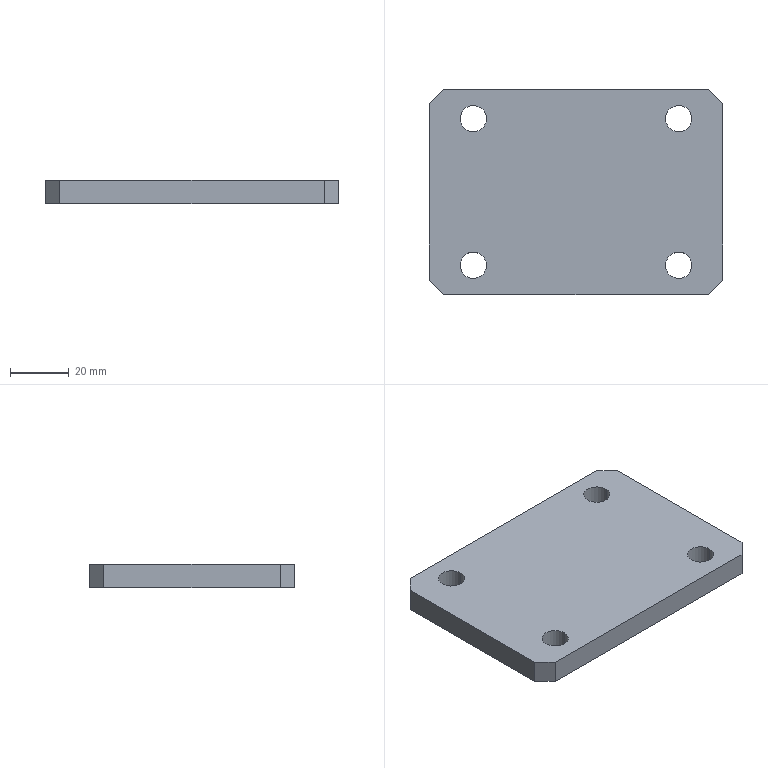Part | SolidWorks | features Chamfer 1, Cut 1, Extrusion 1 | 1 solid | 18 faces | box 100 x 70 x 8 mm | volume 53564 mm3 | plane 10 | cylinder 8 | commonest cylinder face diameters 9 x8
STEP:
#1=CARTESIAN_POINT('',(39.5,-200.,-15.));
#2=VERTEX_POINT('',#1);
#3=CARTESIAN_POINT('',(30.5,-200.,-15.));
#4=VERTEX_POINT('',#3);
#5=CARTESIAN_POINT('',(35.,-200.,-15.));
#6=DIRECTION('',(0.,0.,-1.));
#7=DIRECTION('',(-1.,0.,0.));
#8=AXIS2_PLACEMENT_3D('',#5,#6,#7);
#9=CIRCLE('',#8,4.5);
#10=EDGE_CURVE('',#2,#4,#9,.T.);
#11=ORIENTED_EDGE('',*,*,#10,.F.);
#12=CARTESIAN_POINT('',(39.5,-200.,-23.));
#13=VERTEX_POINT('',#12);
#14=CARTESIAN_POINT('',(39.5,-200.,-15.));
#15=DIRECTION('',(0.,0.,-1.));
#16=VECTOR('',#15,1000.);
#17=LINE('',#14,#16);
#18=EDGE_CURVE('',#2,#13,#17,.T.);
#19=ORIENTED_EDGE('',*,*,#18,.T.);
#20=CARTESIAN_POINT('',(30.5,-200.,-23.));
#21=VERTEX_POINT('',#20);
#22=CARTESIAN_POINT('',(35.,-200.,-23.));
#23=DIRECTION('',(0.,0.,-1.));
#24=DIRECTION('',(-1.,0.,0.));
#25=AXIS2_PLACEMENT_3D('',#22,#23,#24);
#26=CIRCLE('',#25,4.5);
#27=EDGE_CURVE('',#13,#21,#26,.T.);
#28=ORIENTED_EDGE('',*,*,#27,.T.);
#29=CARTESIAN_POINT('',(30.5,-200.,-15.));
#30=DIRECTION('',(0.,0.,-1.));
#31=VECTOR('',#30,1000.);
#32=LINE('',#29,#31);
#33=EDGE_CURVE('',#4,#21,#32,.T.);
#34=ORIENTED_EDGE('',*,*,#33,.F.);
#35=EDGE_LOOP('',(#11,#19,#28,#34));
#36=FACE_OUTER_BOUND('',#35,.T.);
#37=CARTESIAN_POINT('',(35.,-200.,-15.));
#38=DIRECTION('',(0.,0.,-1.));
#39=DIRECTION('',(-1.,0.,0.));
#40=AXIS2_PLACEMENT_3D('',#37,#38,#39);
#41=CYLINDRICAL_SURFACE('',#40,4.5);
#42=ADVANCED_FACE('',(#36),#41,.F.);
#43=CARTESIAN_POINT('',(-30.5,-200.,-15.));
#44=VERTEX_POINT('',#43);
#45=CARTESIAN_POINT('',(-39.5,-200.,-15.));
#46=VERTEX_POINT('',#45);
#47=CARTESIAN_POINT('',(-35.,-200.,-15.));
#48=DIRECTION('',(0.,0.,-1.));
#49=DIRECTION('',(-1.,0.,0.));
#50=AXIS2_PLACEMENT_3D('',#47,#48,#49);
#51=CIRCLE('',#50,4.5);
#52=EDGE_CURVE('',#44,#46,#51,.T.);
#53=ORIENTED_EDGE('',*,*,#52,.F.);
#54=CARTESIAN_POINT('',(-30.5,-200.,-23.));
#55=VERTEX_POINT('',#54);
#56=CARTESIAN_POINT('',(-30.5,-200.,-15.));
#57=DIRECTION('',(0.,0.,-1.));
#58=VECTOR('',#57,1000.);
#59=LINE('',#56,#58);
#60=EDGE_CURVE('',#44,#55,#59,.T.);
#61=ORIENTED_EDGE('',*,*,#60,.T.);
#62=CARTESIAN_POINT('',(-39.5,-200.,-23.));
#63=VERTEX_POINT('',#62);
#64=CARTESIAN_POINT('',(-35.,-200.,-23.));
#65=DIRECTION('',(0.,0.,-1.));
#66=DIRECTION('',(-1.,0.,0.));
#67=AXIS2_PLACEMENT_3D('',#64,#65,#66);
#68=CIRCLE('',#67,4.5);
#69=EDGE_CURVE('',#55,#63,#68,.T.);
#70=ORIENTED_EDGE('',*,*,#69,.T.);
#71=CARTESIAN_POINT('',(-39.5,-200.,-15.));
#72=DIRECTION('',(0.,0.,-1.));
#73=VECTOR('',#72,1000.);
#74=LINE('',#71,#73);
#75=EDGE_CURVE('',#46,#63,#74,.T.);
#76=ORIENTED_EDGE('',*,*,#75,.F.);
#77=EDGE_LOOP('',(#53,#61,#70,#76));
#78=FACE_OUTER_BOUND('',#77,.T.);
#79=CARTESIAN_POINT('',(-35.,-200.,-15.));
#80=DIRECTION('',(0.,0.,-1.));
#81=DIRECTION('',(-1.,0.,0.));
#82=AXIS2_PLACEMENT_3D('',#79,#80,#81);
#83=CYLINDRICAL_SURFACE('',#82,4.5);
#84=ADVANCED_FACE('',(#78),#83,.F.);
#85=CARTESIAN_POINT('',(-30.5,-150.,-15.));
#86=VERTEX_POINT('',#85);
#87=CARTESIAN_POINT('',(-39.5,-150.,-15.));
#88=VERTEX_POINT('',#87);
#89=CARTESIAN_POINT('',(-35.,-150.,-15.));
#90=DIRECTION('',(0.,0.,-1.));
#91=DIRECTION('',(-1.,0.,0.));
#92=AXIS2_PLACEMENT_3D('',#89,#90,#91);
#93=CIRCLE('',#92,4.5);
#94=EDGE_CURVE('',#86,#88,#93,.T.);
#95=ORIENTED_EDGE('',*,*,#94,.F.);
#96=CARTESIAN_POINT('',(-30.5,-150.,-23.));
#97=VERTEX_POINT('',#96);
#98=CARTESIAN_POINT('',(-30.5,-150.,-15.));
#99=DIRECTION('',(0.,0.,-1.));
#100=VECTOR('',#99,1000.);
#101=LINE('',#98,#100);
#102=EDGE_CURVE('',#86,#97,#101,.T.);
#103=ORIENTED_EDGE('',*,*,#102,.T.);
#104=CARTESIAN_POINT('',(-39.5,-150.,-23.));
#105=VERTEX_POINT('',#104);
#106=CARTESIAN_POINT('',(-35.,-150.,-23.));
#107=DIRECTION('',(0.,0.,-1.));
#108=DIRECTION('',(-1.,0.,0.));
#109=AXIS2_PLACEMENT_3D('',#106,#107,#108);
#110=CIRCLE('',#109,4.5);
#111=EDGE_CURVE('',#97,#105,#110,.T.);
#112=ORIENTED_EDGE('',*,*,#111,.T.);
#113=CARTESIAN_POINT('',(-39.5,-150.,-15.));
#114=DIRECTION('',(0.,0.,-1.));
#115=VECTOR('',#114,1000.);
#116=LINE('',#113,#115);
#117=EDGE_CURVE('',#88,#105,#116,.T.);
#118=ORIENTED_EDGE('',*,*,#117,.F.);
#119=EDGE_LOOP('',(#95,#103,#112,#118));
#120=FACE_OUTER_BOUND('',#119,.T.);
#121=CARTESIAN_POINT('',(-35.,-150.,-15.));
#122=DIRECTION('',(0.,0.,-1.));
#123=DIRECTION('',(-1.,0.,0.));
#124=AXIS2_PLACEMENT_3D('',#121,#122,#123);
#125=CYLINDRICAL_SURFACE('',#124,4.5);
#126=ADVANCED_FACE('',(#120),#125,.F.);
#127=CARTESIAN_POINT('',(39.5,-150.,-15.));
#128=VERTEX_POINT('',#127);
#129=CARTESIAN_POINT('',(30.5,-150.,-15.));
#130=VERTEX_POINT('',#129);
#131=CARTESIAN_POINT('',(35.,-150.,-15.));
#132=DIRECTION('',(0.,0.,-1.));
#133=DIRECTION('',(-1.,0.,0.));
#134=AXIS2_PLACEMENT_3D('',#131,#132,#133);
#135=CIRCLE('',#134,4.5);
#136=EDGE_CURVE('',#128,#130,#135,.T.);
#137=ORIENTED_EDGE('',*,*,#136,.F.);
#138=CARTESIAN_POINT('',(39.5,-150.,-23.));
#139=VERTEX_POINT('',#138);
#140=CARTESIAN_POINT('',(39.5,-150.,-15.));
#141=DIRECTION('',(0.,0.,-1.));
#142=VECTOR('',#141,1000.);
#143=LINE('',#140,#142);
#144=EDGE_CURVE('',#128,#139,#143,.T.);
#145=ORIENTED_EDGE('',*,*,#144,.T.);
#146=CARTESIAN_POINT('',(30.5,-150.,-23.));
#147=VERTEX_POINT('',#146);
#148=CARTESIAN_POINT('',(35.,-150.,-23.));
#149=DIRECTION('',(0.,0.,-1.));
#150=DIRECTION('',(-1.,0.,0.));
#151=AXIS2_PLACEMENT_3D('',#148,#149,#150);
#152=CIRCLE('',#151,4.5);
#153=EDGE_CURVE('',#139,#147,#152,.T.);
#154=ORIENTED_EDGE('',*,*,#153,.T.);
#155=CARTESIAN_POINT('',(30.5,-150.,-15.));
#156=DIRECTION('',(0.,0.,-1.));
#157=VECTOR('',#156,1000.);
#158=LINE('',#155,#157);
#159=EDGE_CURVE('',#130,#147,#158,.T.);
#160=ORIENTED_EDGE('',*,*,#159,.F.);
#161=EDGE_LOOP('',(#137,#145,#154,#160));
#162=FACE_OUTER_BOUND('',#161,.T.);
#163=CARTESIAN_POINT('',(35.,-150.,-15.));
#164=DIRECTION('',(0.,0.,-1.));
#165=DIRECTION('',(-1.,0.,0.));
#166=AXIS2_PLACEMENT_3D('',#163,#164,#165);
#167=CYLINDRICAL_SURFACE('',#166,4.5);
#168=ADVANCED_FACE('',(#162),#167,.F.);
#169=CARTESIAN_POINT('',(50.,-205.,-23.));
#170=VERTEX_POINT('',#169);
#171=CARTESIAN_POINT('',(50.,-145.,-23.));
#172=VERTEX_POINT('',#171);
#173=CARTESIAN_POINT('',(50.,-140.,-23.));
#174=DIRECTION('',(0.,1.,0.));
#175=VECTOR('',#174,1000.);
#176=LINE('',#173,#175);
#177=EDGE_CURVE('',#170,#172,#176,.T.);
#178=ORIENTED_EDGE('',*,*,#177,.T.);
#179=CARTESIAN_POINT('',(50.,-145.,-15.));
#180=VERTEX_POINT('',#179);
#181=CARTESIAN_POINT('',(50.,-145.,-23.));
#182=DIRECTION('',(0.,0.,1.));
#183=VECTOR('',#182,1000.);
#184=LINE('',#181,#183);
#185=EDGE_CURVE('',#172,#180,#184,.T.);
#186=ORIENTED_EDGE('',*,*,#185,.T.);
#187=CARTESIAN_POINT('',(50.,-205.,-15.));
#188=VERTEX_POINT('',#187);
#189=CARTESIAN_POINT('',(50.,-140.,-15.));
#190=DIRECTION('',(0.,1.,0.));
#191=VECTOR('',#190,1000.);
#192=LINE('',#189,#191);
#193=EDGE_CURVE('',#188,#180,#192,.T.);
#194=ORIENTED_EDGE('',*,*,#193,.F.);
#195=CARTESIAN_POINT('',(50.,-205.,-23.));
#196=DIRECTION('',(0.,0.,-1.));
#197=VECTOR('',#196,1000.);
#198=LINE('',#195,#197);
#199=EDGE_CURVE('',#188,#170,#198,.T.);
#200=ORIENTED_EDGE('',*,*,#199,.T.);
#201=EDGE_LOOP('',(#178,#186,#194,#200));
#202=FACE_OUTER_BOUND('',#201,.T.);
#203=CARTESIAN_POINT('',(50.,-140.,-23.));
#204=DIRECTION('',(1.,0.,0.));
#205=DIRECTION('',(0.,1.,0.));
#206=AXIS2_PLACEMENT_3D('',#203,#204,#205);
#207=PLANE('',#206);
#208=ADVANCED_FACE('',(#202),#207,.T.);
#209=CARTESIAN_POINT('',(-45.,-210.,-15.));
#210=VERTEX_POINT('',#209);
#211=CARTESIAN_POINT('',(45.,-210.,-15.));
#212=VERTEX_POINT('',#211);
#213=CARTESIAN_POINT('',(-50.,-210.,-15.));
#214=DIRECTION('',(1.,0.,0.));
#215=VECTOR('',#214,1000.);
#216=LINE('',#213,#215);
#217=EDGE_CURVE('',#210,#212,#216,.T.);
#218=ORIENTED_EDGE('',*,*,#217,.F.);
#219=CARTESIAN_POINT('',(-45.,-210.,-23.));
#220=VERTEX_POINT('',#219);
#221=CARTESIAN_POINT('',(-45.,-210.,-23.));
#222=DIRECTION('',(0.,0.,-1.));
#223=VECTOR('',#222,1000.);
#224=LINE('',#221,#223);
#225=EDGE_CURVE('',#210,#220,#224,.T.);
#226=ORIENTED_EDGE('',*,*,#225,.T.);
#227=CARTESIAN_POINT('',(45.,-210.,-23.));
#228=VERTEX_POINT('',#227);
#229=CARTESIAN_POINT('',(-50.,-210.,-23.));
#230=DIRECTION('',(1.,0.,0.));
#231=VECTOR('',#230,1000.);
#232=LINE('',#229,#231);
#233=EDGE_CURVE('',#220,#228,#232,.T.);
#234=ORIENTED_EDGE('',*,*,#233,.T.);
#235=CARTESIAN_POINT('',(45.,-210.,-23.));
#236=DIRECTION('',(0.,0.,1.));
#237=VECTOR('',#236,1000.);
#238=LINE('',#235,#237);
#239=EDGE_CURVE('',#228,#212,#238,.T.);
#240=ORIENTED_EDGE('',*,*,#239,.T.);
#241=EDGE_LOOP('',(#218,#226,#234,#240));
#242=FACE_OUTER_BOUND('',#241,.T.);
#243=CARTESIAN_POINT('',(-50.,-210.,-23.));
#244=DIRECTION('',(0.,-1.,0.));
#245=DIRECTION('',(0.,0.,-1.));
#246=AXIS2_PLACEMENT_3D('',#243,#244,#245);
#247=PLANE('',#246);
#248=ADVANCED_FACE('',(#242),#247,.T.);
#249=CARTESIAN_POINT('',(-50.,-145.,-15.));
#250=VERTEX_POINT('',#249);
#251=CARTESIAN_POINT('',(-50.,-205.,-15.));
#252=VERTEX_POINT('',#251);
#253=CARTESIAN_POINT('',(-50.,-140.,-15.));
#254=DIRECTION('',(0.,-1.,0.));
#255=VECTOR('',#254,1000.);
#256=LINE('',#253,#255);
#257=EDGE_CURVE('',#250,#252,#256,.T.);
#258=ORIENTED_EDGE('',*,*,#257,.F.);
#259=CARTESIAN_POINT('',(-50.,-145.,-23.));
#260=VERTEX_POINT('',#259);
#261=CARTESIAN_POINT('',(-50.,-145.,-23.));
#262=DIRECTION('',(0.,0.,-1.));
#263=VECTOR('',#262,1000.);
#264=LINE('',#261,#263);
#265=EDGE_CURVE('',#250,#260,#264,.T.);
#266=ORIENTED_EDGE('',*,*,#265,.T.);
#267=CARTESIAN_POINT('',(-50.,-205.,-23.));
#268=VERTEX_POINT('',#267);
#269=CARTESIAN_POINT('',(-50.,-140.,-23.));
#270=DIRECTION('',(0.,-1.,0.));
#271=VECTOR('',#270,1000.);
#272=LINE('',#269,#271);
#273=EDGE_CURVE('',#260,#268,#272,.T.);
#274=ORIENTED_EDGE('',*,*,#273,.T.);
#275=CARTESIAN_POINT('',(-50.,-205.,-23.));
#276=DIRECTION('',(0.,0.,1.));
#277=VECTOR('',#276,1000.);
#278=LINE('',#275,#277);
#279=EDGE_CURVE('',#268,#252,#278,.T.);
#280=ORIENTED_EDGE('',*,*,#279,.T.);
#281=EDGE_LOOP('',(#258,#266,#274,#280));
#282=FACE_OUTER_BOUND('',#281,.T.);
#283=CARTESIAN_POINT('',(-50.,-140.,-23.));
#284=DIRECTION('',(-1.,0.,0.));
#285=DIRECTION('',(0.,-1.,0.));
#286=AXIS2_PLACEMENT_3D('',#283,#284,#285);
#287=PLANE('',#286);
#288=ADVANCED_FACE('',(#282),#287,.T.);
#289=CARTESIAN_POINT('',(45.,-140.,-23.));
#290=VERTEX_POINT('',#289);
#291=CARTESIAN_POINT('',(-45.,-140.,-23.));
#292=VERTEX_POINT('',#291);
#293=CARTESIAN_POINT('',(-50.,-140.,-23.));
#294=DIRECTION('',(-1.,0.,0.));
#295=VECTOR('',#294,1000.);
#296=LINE('',#293,#295);
#297=EDGE_CURVE('',#290,#292,#296,.T.);
#298=ORIENTED_EDGE('',*,*,#297,.T.);
#299=CARTESIAN_POINT('',(-45.,-140.,-15.));
#300=VERTEX_POINT('',#299);
#301=CARTESIAN_POINT('',(-45.,-140.,-23.));
#302=DIRECTION('',(0.,0.,1.));
#303=VECTOR('',#302,1000.);
#304=LINE('',#301,#303);
#305=EDGE_CURVE('',#292,#300,#304,.T.);
#306=ORIENTED_EDGE('',*,*,#305,.T.);
#307=CARTESIAN_POINT('',(45.,-140.,-15.));
#308=VERTEX_POINT('',#307);
#309=CARTESIAN_POINT('',(-50.,-140.,-15.));
#310=DIRECTION('',(-1.,0.,0.));
#311=VECTOR('',#310,1000.);
#312=LINE('',#309,#311);
#313=EDGE_CURVE('',#308,#300,#312,.T.);
#314=ORIENTED_EDGE('',*,*,#313,.F.);
#315=CARTESIAN_POINT('',(45.,-140.,-23.));
#316=DIRECTION('',(0.,0.,-1.));
#317=VECTOR('',#316,1000.);
#318=LINE('',#315,#317);
#319=EDGE_CURVE('',#308,#290,#318,.T.);
#320=ORIENTED_EDGE('',*,*,#319,.T.);
#321=EDGE_LOOP('',(#298,#306,#314,#320));
#322=FACE_OUTER_BOUND('',#321,.T.);
#323=CARTESIAN_POINT('',(-50.,-140.,-23.));
#324=DIRECTION('',(0.,1.,0.));
#325=DIRECTION('',(-1.,0.,0.));
#326=AXIS2_PLACEMENT_3D('',#323,#324,#325);
#327=PLANE('',#326);
#328=ADVANCED_FACE('',(#322),#327,.T.);
#329=CARTESIAN_POINT('',(35.,-200.,-23.));
#330=DIRECTION('',(0.,0.,-1.));
#331=DIRECTION('',(-1.,0.,0.));
#332=AXIS2_PLACEMENT_3D('',#329,#330,#331);
#333=CIRCLE('',#332,4.5);
#334=EDGE_CURVE('',#21,#13,#333,.T.);
#335=ORIENTED_EDGE('',*,*,#334,.F.);
#336=ORIENTED_EDGE('',*,*,#27,.F.);
#337=EDGE_LOOP('',(#335,#336));
#338=FACE_BOUND('',#337,.T.);
#339=CARTESIAN_POINT('',(-35.,-200.,-23.));
#340=DIRECTION('',(0.,0.,-1.));
#341=DIRECTION('',(-1.,0.,0.));
#342=AXIS2_PLACEMENT_3D('',#339,#340,#341);
#343=CIRCLE('',#342,4.5);
#344=EDGE_CURVE('',#63,#55,#343,.T.);
#345=ORIENTED_EDGE('',*,*,#344,.F.);
#346=ORIENTED_EDGE('',*,*,#69,.F.);
#347=EDGE_LOOP('',(#345,#346));
#348=FACE_BOUND('',#347,.T.);
#349=CARTESIAN_POINT('',(-35.,-150.,-23.));
#350=DIRECTION('',(0.,0.,-1.));
#351=DIRECTION('',(-1.,0.,0.));
#352=AXIS2_PLACEMENT_3D('',#349,#350,#351);
#353=CIRCLE('',#352,4.5);
#354=EDGE_CURVE('',#105,#97,#353,.T.);
#355=ORIENTED_EDGE('',*,*,#354,.F.);
#356=ORIENTED_EDGE('',*,*,#111,.F.);
#357=EDGE_LOOP('',(#355,#356));
#358=FACE_BOUND('',#357,.T.);
#359=CARTESIAN_POINT('',(35.,-150.,-23.));
#360=DIRECTION('',(0.,0.,-1.));
#361=DIRECTION('',(-1.,0.,0.));
#362=AXIS2_PLACEMENT_3D('',#359,#360,#361);
#363=CIRCLE('',#362,4.5);
#364=EDGE_CURVE('',#147,#139,#363,.T.);
#365=ORIENTED_EDGE('',*,*,#364,.F.);
#366=ORIENTED_EDGE('',*,*,#153,.F.);
#367=EDGE_LOOP('',(#365,#366));
#368=FACE_BOUND('',#367,.T.);
#369=ORIENTED_EDGE('',*,*,#273,.F.);
#370=CARTESIAN_POINT('',(-45.,-140.,-23.));
#371=DIRECTION('',(0.7071,0.7071,0.));
#372=VECTOR('',#371,1000.);
#373=LINE('',#370,#372);
#374=EDGE_CURVE('',#260,#292,#373,.T.);
#375=ORIENTED_EDGE('',*,*,#374,.T.);
#376=ORIENTED_EDGE('',*,*,#297,.F.);
#377=CARTESIAN_POINT('',(50.,-145.,-23.));
#378=DIRECTION('',(0.7071,-0.7071,0.));
#379=VECTOR('',#378,1000.);
#380=LINE('',#377,#379);
#381=EDGE_CURVE('',#290,#172,#380,.T.);
#382=ORIENTED_EDGE('',*,*,#381,.T.);
#383=ORIENTED_EDGE('',*,*,#177,.F.);
#384=CARTESIAN_POINT('',(45.,-210.,-23.));
#385=DIRECTION('',(-0.7071,-0.7071,0.));
#386=VECTOR('',#385,1000.);
#387=LINE('',#384,#386);
#388=EDGE_CURVE('',#170,#228,#387,.T.);
#389=ORIENTED_EDGE('',*,*,#388,.T.);
#390=ORIENTED_EDGE('',*,*,#233,.F.);
#391=CARTESIAN_POINT('',(-50.,-205.,-23.));
#392=DIRECTION('',(-0.7071,0.7071,0.));
#393=VECTOR('',#392,1000.);
#394=LINE('',#391,#393);
#395=EDGE_CURVE('',#220,#268,#394,.T.);
#396=ORIENTED_EDGE('',*,*,#395,.T.);
#397=EDGE_LOOP('',(#369,#375,#376,#382,#383,#389,#390,#396));
#398=FACE_OUTER_BOUND('',#397,.T.);
#399=CARTESIAN_POINT('',(0.,0.,-23.));
#400=DIRECTION('',(0.,0.,1.));
#401=DIRECTION('',(1.,0.,0.));
#402=AXIS2_PLACEMENT_3D('',#399,#400,#401);
#403=PLANE('',#402);
#404=ADVANCED_FACE('',(#338,#348,#358,#368,#398),#403,.F.);
#405=CARTESIAN_POINT('',(35.,-200.,-15.));
#406=DIRECTION('',(0.,0.,-1.));
#407=DIRECTION('',(-1.,0.,0.));
#408=AXIS2_PLACEMENT_3D('',#405,#406,#407);
#409=CIRCLE('',#408,4.5);
#410=EDGE_CURVE('',#4,#2,#409,.T.);
#411=ORIENTED_EDGE('',*,*,#410,.T.);
#412=ORIENTED_EDGE('',*,*,#10,.T.);
#413=EDGE_LOOP('',(#411,#412));
#414=FACE_BOUND('',#413,.T.);
#415=CARTESIAN_POINT('',(-35.,-200.,-15.));
#416=DIRECTION('',(0.,0.,-1.));
#417=DIRECTION('',(-1.,0.,0.));
#418=AXIS2_PLACEMENT_3D('',#415,#416,#417);
#419=CIRCLE('',#418,4.5);
#420=EDGE_CURVE('',#46,#44,#419,.T.);
#421=ORIENTED_EDGE('',*,*,#420,.T.);
#422=ORIENTED_EDGE('',*,*,#52,.T.);
#423=EDGE_LOOP('',(#421,#422));
#424=FACE_BOUND('',#423,.T.);
#425=CARTESIAN_POINT('',(-35.,-150.,-15.));
#426=DIRECTION('',(0.,0.,-1.));
#427=DIRECTION('',(-1.,0.,0.));
#428=AXIS2_PLACEMENT_3D('',#425,#426,#427);
#429=CIRCLE('',#428,4.5);
#430=EDGE_CURVE('',#88,#86,#429,.T.);
#431=ORIENTED_EDGE('',*,*,#430,.T.);
#432=ORIENTED_EDGE('',*,*,#94,.T.);
#433=EDGE_LOOP('',(#431,#432));
#434=FACE_BOUND('',#433,.T.);
#435=CARTESIAN_POINT('',(35.,-150.,-15.));
#436=DIRECTION('',(0.,0.,-1.));
#437=DIRECTION('',(-1.,0.,0.));
#438=AXIS2_PLACEMENT_3D('',#435,#436,#437);
#439=CIRCLE('',#438,4.5);
#440=EDGE_CURVE('',#130,#128,#439,.T.);
#441=ORIENTED_EDGE('',*,*,#440,.T.);
#442=ORIENTED_EDGE('',*,*,#136,.T.);
#443=EDGE_LOOP('',(#441,#442));
#444=FACE_BOUND('',#443,.T.);
#445=ORIENTED_EDGE('',*,*,#313,.T.);
#446=CARTESIAN_POINT('',(47.5,-47.5,-15.));
#447=DIRECTION('',(-0.7071,-0.7071,0.));
#448=VECTOR('',#447,1000.);
#449=LINE('',#446,#448);
#450=EDGE_CURVE('',#300,#250,#449,.T.);
#451=ORIENTED_EDGE('',*,*,#450,.T.);
#452=ORIENTED_EDGE('',*,*,#257,.T.);
#453=CARTESIAN_POINT('',(-127.5,-127.5,-15.));
#454=DIRECTION('',(0.7071,-0.7071,0.));
#455=VECTOR('',#454,1000.);
#456=LINE('',#453,#455);
#457=EDGE_CURVE('',#252,#210,#456,.T.);
#458=ORIENTED_EDGE('',*,*,#457,.T.);
#459=ORIENTED_EDGE('',*,*,#217,.T.);
#460=CARTESIAN_POINT('',(127.5,-127.5,-15.));
#461=DIRECTION('',(0.7071,0.7071,0.));
#462=VECTOR('',#461,1000.);
#463=LINE('',#460,#462);
#464=EDGE_CURVE('',#212,#188,#463,.T.);
#465=ORIENTED_EDGE('',*,*,#464,.T.);
#466=ORIENTED_EDGE('',*,*,#193,.T.);
#467=CARTESIAN_POINT('',(-47.5,-47.5,-15.));
#468=DIRECTION('',(-0.7071,0.7071,0.));
#469=VECTOR('',#468,1000.);
#470=LINE('',#467,#469);
#471=EDGE_CURVE('',#180,#308,#470,.T.);
#472=ORIENTED_EDGE('',*,*,#471,.T.);
#473=EDGE_LOOP('',(#445,#451,#452,#458,#459,#465,#466,#472));
#474=FACE_OUTER_BOUND('',#473,.T.);
#475=CARTESIAN_POINT('',(0.,0.,-15.));
#476=DIRECTION('',(0.,0.,1.));
#477=DIRECTION('',(1.,0.,0.));
#478=AXIS2_PLACEMENT_3D('',#475,#476,#477);
#479=PLANE('',#478);
#480=ADVANCED_FACE('',(#414,#424,#434,#444,#474),#479,.T.);
#481=ORIENTED_EDGE('',*,*,#144,.F.);
#482=ORIENTED_EDGE('',*,*,#440,.F.);
#483=ORIENTED_EDGE('',*,*,#159,.T.);
#484=ORIENTED_EDGE('',*,*,#364,.T.);
#485=EDGE_LOOP('',(#481,#482,#483,#484));
#486=FACE_OUTER_BOUND('',#485,.T.);
#487=CARTESIAN_POINT('',(35.,-150.,-15.));
#488=DIRECTION('',(0.,0.,-1.));
#489=DIRECTION('',(-1.,0.,0.));
#490=AXIS2_PLACEMENT_3D('',#487,#488,#489);
#491=CYLINDRICAL_SURFACE('',#490,4.5);
#492=ADVANCED_FACE('',(#486),#491,.F.);
#493=ORIENTED_EDGE('',*,*,#102,.F.);
#494=ORIENTED_EDGE('',*,*,#430,.F.);
#495=ORIENTED_EDGE('',*,*,#117,.T.);
#496=ORIENTED_EDGE('',*,*,#354,.T.);
#497=EDGE_LOOP('',(#493,#494,#495,#496));
#498=FACE_OUTER_BOUND('',#497,.T.);
#499=CARTESIAN_POINT('',(-35.,-150.,-15.));
#500=DIRECTION('',(0.,0.,-1.));
#501=DIRECTION('',(-1.,0.,0.));
#502=AXIS2_PLACEMENT_3D('',#499,#500,#501);
#503=CYLINDRICAL_SURFACE('',#502,4.5);
#504=ADVANCED_FACE('',(#498),#503,.F.);
#505=ORIENTED_EDGE('',*,*,#60,.F.);
#506=ORIENTED_EDGE('',*,*,#420,.F.);
#507=ORIENTED_EDGE('',*,*,#75,.T.);
#508=ORIENTED_EDGE('',*,*,#344,.T.);
#509=EDGE_LOOP('',(#505,#506,#507,#508));
#510=FACE_OUTER_BOUND('',#509,.T.);
#511=CARTESIAN_POINT('',(-35.,-200.,-15.));
#512=DIRECTION('',(0.,0.,-1.));
#513=DIRECTION('',(-1.,0.,0.));
#514=AXIS2_PLACEMENT_3D('',#511,#512,#513);
#515=CYLINDRICAL_SURFACE('',#514,4.5);
#516=ADVANCED_FACE('',(#510),#515,.F.);
#517=ORIENTED_EDGE('',*,*,#18,.F.);
#518=ORIENTED_EDGE('',*,*,#410,.F.);
#519=ORIENTED_EDGE('',*,*,#33,.T.);
#520=ORIENTED_EDGE('',*,*,#334,.T.);
#521=EDGE_LOOP('',(#517,#518,#519,#520));
#522=FACE_OUTER_BOUND('',#521,.T.);
#523=CARTESIAN_POINT('',(35.,-200.,-15.));
#524=DIRECTION('',(0.,0.,-1.));
#525=DIRECTION('',(-1.,0.,0.));
#526=AXIS2_PLACEMENT_3D('',#523,#524,#525);
#527=CYLINDRICAL_SURFACE('',#526,4.5);
#528=ADVANCED_FACE('',(#522),#527,.F.);
#529=ORIENTED_EDGE('',*,*,#374,.F.);
#530=ORIENTED_EDGE('',*,*,#265,.F.);
#531=ORIENTED_EDGE('',*,*,#450,.F.);
#532=ORIENTED_EDGE('',*,*,#305,.F.);
#533=EDGE_LOOP('',(#529,#530,#531,#532));
#534=FACE_OUTER_BOUND('',#533,.T.);
#535=CARTESIAN_POINT('',(-45.,-140.,-23.));
#536=DIRECTION('',(0.7071,-0.7071,0.));
#537=DIRECTION('',(0.,0.,1.));
#538=AXIS2_PLACEMENT_3D('',#535,#536,#537);
#539=PLANE('',#538);
#540=ADVANCED_FACE('',(#534),#539,.F.);
#541=ORIENTED_EDGE('',*,*,#395,.F.);
#542=ORIENTED_EDGE('',*,*,#225,.F.);
#543=ORIENTED_EDGE('',*,*,#457,.F.);
#544=ORIENTED_EDGE('',*,*,#279,.F.);
#545=EDGE_LOOP('',(#541,#542,#543,#544));
#546=FACE_OUTER_BOUND('',#545,.T.);
#547=CARTESIAN_POINT('',(-50.,-205.,-23.));
#548=DIRECTION('',(0.7071,0.7071,0.));
#549=DIRECTION('',(0.,0.,1.));
#550=AXIS2_PLACEMENT_3D('',#547,#548,#549);
#551=PLANE('',#550);
#552=ADVANCED_FACE('',(#546),#551,.F.);
#553=ORIENTED_EDGE('',*,*,#381,.F.);
#554=ORIENTED_EDGE('',*,*,#319,.F.);
#555=ORIENTED_EDGE('',*,*,#471,.F.);
#556=ORIENTED_EDGE('',*,*,#185,.F.);
#557=EDGE_LOOP('',(#553,#554,#555,#556));
#558=FACE_OUTER_BOUND('',#557,.T.);
#559=CARTESIAN_POINT('',(50.,-145.,-23.));
#560=DIRECTION('',(-0.7071,-0.7071,0.));
#561=DIRECTION('',(0.,0.,1.));
#562=AXIS2_PLACEMENT_3D('',#559,#560,#561);
#563=PLANE('',#562);
#564=ADVANCED_FACE('',(#558),#563,.F.);
#565=ORIENTED_EDGE('',*,*,#388,.F.);
#566=ORIENTED_EDGE('',*,*,#199,.F.);
#567=ORIENTED_EDGE('',*,*,#464,.F.);
#568=ORIENTED_EDGE('',*,*,#239,.F.);
#569=EDGE_LOOP('',(#565,#566,#567,#568));
#570=FACE_OUTER_BOUND('',#569,.T.);
#571=CARTESIAN_POINT('',(45.,-210.,-23.));
#572=DIRECTION('',(-0.7071,0.7071,0.));
#573=DIRECTION('',(0.,0.,1.));
#574=AXIS2_PLACEMENT_3D('',#571,#572,#573);
#575=PLANE('',#574);
#576=ADVANCED_FACE('',(#570),#575,.F.);
#577=CLOSED_SHELL('',(#42,#84,#126,#168,#208,#248,#288,#328,#404,#480,#492,#504,#516,#528,#540,#552,#564,#576));
#578=MANIFOLD_SOLID_BREP('',#577);
#579=CARTESIAN_POINT('',(0.,0.,0.));
#580=DIRECTION('',(0.,0.,1.));
#581=DIRECTION('',(1.,0.,0.));
#582=AXIS2_PLACEMENT_3D('',#579,#580,#581);
#583=(LENGTH_UNIT()NAMED_UNIT(*)SI_UNIT(.MILLI.,.METRE.));
#584=UNCERTAINTY_MEASURE_WITH_UNIT(LENGTH_MEASURE(0.00001),#583,'','');
#585=(NAMED_UNIT(*)PLANE_ANGLE_UNIT()SI_UNIT($,.RADIAN.));
#586=(NAMED_UNIT(*)SI_UNIT($,.STERADIAN.)SOLID_ANGLE_UNIT());
#587=(GEOMETRIC_REPRESENTATION_CONTEXT(3)GLOBAL_UNCERTAINTY_ASSIGNED_CONTEXT((#584))GLOBAL_UNIT_ASSIGNED_CONTEXT((#583,#585,#586))REPRESENTATION_CONTEXT('',''));
#588=ADVANCED_BREP_SHAPE_REPRESENTATION('',(#578,#582),#587);